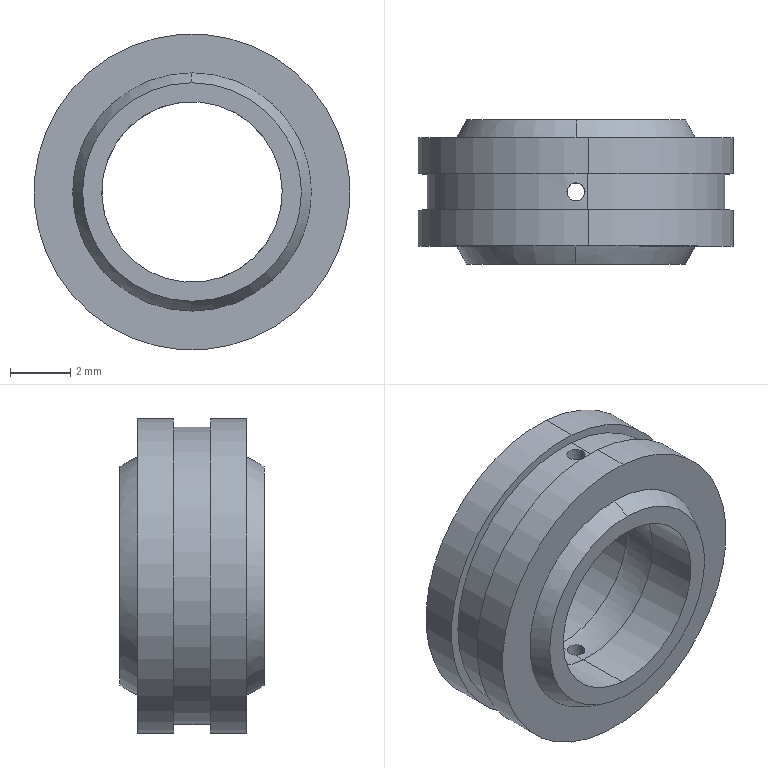Part | STEP file | 2026.6.15-Main Assembly图.sldasm-Part-227 | 1 solid | 29 faces | box 10.5 x 4.8 x 10.5 mm | volume 217.629 mm3 | cylinder 14 | plane 6 | torus 5 | sphere 4 | commonest cylinder face diameters 0.6 x4 6 x4 10.5 x4 9.9 x2
STEP:
#1=CARTESIAN_POINT('',(-1513.188,1424.864,3411.086));
#2=VERTEX_POINT('',#1);
#3=CARTESIAN_POINT('',(-1513.424,1424.864,3405.096));
#4=VERTEX_POINT('',#3);
#5=CARTESIAN_POINT('',(-1513.188,1424.864,3408.086));
#6=DIRECTION('',(0.,-1.,0.));
#7=DIRECTION('',(0.0785,0.,0.9969));
#8=AXIS2_PLACEMENT_3D('',#5,#6,#7);
#9=CIRCLE('',#8,3.);
#10=EDGE_CURVE('',#2,#4,#9,.T.);
#11=ORIENTED_EDGE('',*,*,#10,.F.);
#12=CARTESIAN_POINT('',(-1513.188,1424.564,3411.104));
#13=VERTEX_POINT('',#12);
#14=CARTESIAN_POINT('',(-1513.188,1424.264,3403.323));
#15=DIRECTION('',(1.,0.,0.));
#16=DIRECTION('',(0.,1.,0.));
#17=AXIS2_PLACEMENT_3D('',#14,#15,#16);
#18=CIRCLE('',#17,7.786);
#19=EDGE_CURVE('',#2,#13,#18,.T.);
#20=ORIENTED_EDGE('',*,*,#19,.T.);
#21=CARTESIAN_POINT('',(-1513.488,1424.264,3411.095));
#22=VERTEX_POINT('',#21);
#23=CARTESIAN_POINT('',(-1513.188,1424.564,3411.104));
#24=CARTESIAN_POINT('',(-1513.267,1424.564,3411.104));
#25=CARTESIAN_POINT('',(-1513.344,1424.532,3411.102));
#26=CARTESIAN_POINT('',(-1513.456,1424.421,3411.097));
#27=CARTESIAN_POINT('',(-1513.488,1424.344,3411.095));
#28=CARTESIAN_POINT('',(-1513.488,1424.264,3411.095));
#29=B_SPLINE_CURVE_WITH_KNOTS('',3,(#23,#24,#25,#26,#27,#28),.UNSPECIFIED.,.F.,.F.,(4,2,4),(0.0002723,0.0005067,0.0007411),.UNSPECIFIED.);
#30=EDGE_CURVE('',#13,#22,#29,.T.);
#31=ORIENTED_EDGE('',*,*,#30,.T.);
#32=CARTESIAN_POINT('',(-1513.188,1423.964,3411.104));
#33=VERTEX_POINT('',#32);
#34=CARTESIAN_POINT('',(-1513.488,1424.264,3411.095));
#35=CARTESIAN_POINT('',(-1513.488,1424.185,3411.095));
#36=CARTESIAN_POINT('',(-1513.456,1424.107,3411.097));
#37=CARTESIAN_POINT('',(-1513.345,1423.997,3411.102));
#38=CARTESIAN_POINT('',(-1513.267,1423.964,3411.104));
#39=CARTESIAN_POINT('',(-1513.188,1423.964,3411.104));
#40=B_SPLINE_CURVE_WITH_KNOTS('',3,(#34,#35,#36,#37,#38,#39),.UNSPECIFIED.,.F.,.F.,(4,2,4),(0.,0.0002346,0.0004692),.UNSPECIFIED.);
#41=EDGE_CURVE('',#22,#33,#40,.T.);
#42=ORIENTED_EDGE('',*,*,#41,.T.);
#43=CARTESIAN_POINT('',(-1513.188,1423.664,3411.086));
#44=VERTEX_POINT('',#43);
#45=CARTESIAN_POINT('',(-1513.188,1424.264,3403.323));
#46=DIRECTION('',(1.,0.,0.));
#47=DIRECTION('',(0.,1.,0.));
#48=AXIS2_PLACEMENT_3D('',#45,#46,#47);
#49=CIRCLE('',#48,7.786);
#50=EDGE_CURVE('',#33,#44,#49,.T.);
#51=ORIENTED_EDGE('',*,*,#50,.T.);
#52=CARTESIAN_POINT('',(-1513.424,1423.664,3405.096));
#53=VERTEX_POINT('',#52);
#54=CARTESIAN_POINT('',(-1513.188,1423.664,3408.086));
#55=DIRECTION('',(0.,-1.,0.));
#56=DIRECTION('',(-0.0785,0.,-0.9969));
#57=AXIS2_PLACEMENT_3D('',#54,#55,#56);
#58=CIRCLE('',#57,3.);
#59=EDGE_CURVE('',#44,#53,#58,.T.);
#60=ORIENTED_EDGE('',*,*,#59,.T.);
#61=CARTESIAN_POINT('',(-1513.425,1424.081,3405.075));
#62=VERTEX_POINT('',#61);
#63=CARTESIAN_POINT('',(-1512.814,1424.264,3412.835));
#64=DIRECTION('',(-0.9969,0.,0.0785));
#65=DIRECTION('',(-0.0785,0.,-0.9969));
#66=AXIS2_PLACEMENT_3D('',#63,#64,#65);
#67=CIRCLE('',#66,7.786);
#68=EDGE_CURVE('',#62,#53,#67,.T.);
#69=ORIENTED_EDGE('',*,*,#68,.F.);
#70=CARTESIAN_POINT('',(-1513.488,1424.264,3405.078));
#71=VERTEX_POINT('',#70);
#72=CARTESIAN_POINT('',(-1513.425,1424.081,3405.075));
#73=CARTESIAN_POINT('',(-1513.466,1424.133,3405.077));
#74=CARTESIAN_POINT('',(-1513.488,1424.198,3405.078));
#75=CARTESIAN_POINT('',(-1513.488,1424.264,3405.078));
#76=B_SPLINE_CURVE_WITH_KNOTS('',3,(#72,#73,#74,#75),.UNSPECIFIED.,.F.,.F.,(4,4),(0.,0.0001968),.UNSPECIFIED.);
#77=EDGE_CURVE('',#62,#71,#76,.T.);
#78=ORIENTED_EDGE('',*,*,#77,.T.);
#79=CARTESIAN_POINT('',(-1513.425,1424.448,3405.075));
#80=VERTEX_POINT('',#79);
#81=CARTESIAN_POINT('',(-1513.488,1424.264,3405.078));
#82=CARTESIAN_POINT('',(-1513.488,1424.331,3405.078));
#83=CARTESIAN_POINT('',(-1513.466,1424.395,3405.077));
#84=CARTESIAN_POINT('',(-1513.425,1424.448,3405.075));
#85=B_SPLINE_CURVE_WITH_KNOTS('',3,(#81,#82,#83,#84),.UNSPECIFIED.,.F.,.F.,(4,4),(0.,0.0001968),.UNSPECIFIED.);
#86=EDGE_CURVE('',#71,#80,#85,.T.);
#87=ORIENTED_EDGE('',*,*,#86,.T.);
#88=CARTESIAN_POINT('',(-1512.814,1424.264,3412.835));
#89=DIRECTION('',(-0.9969,0.,0.0785));
#90=DIRECTION('',(-0.0785,0.,-0.9969));
#91=AXIS2_PLACEMENT_3D('',#88,#89,#90);
#92=CIRCLE('',#91,7.786);
#93=EDGE_CURVE('',#4,#80,#92,.T.);
#94=ORIENTED_EDGE('',*,*,#93,.F.);
#95=EDGE_LOOP('',(#11,#20,#31,#42,#51,#60,#69,#78,#87,#94));
#96=FACE_OUTER_BOUND('',#95,.T.);
#97=CARTESIAN_POINT('',(-1513.188,1424.264,3408.086));
#98=DIRECTION('',(0.,-1.,0.));
#99=DIRECTION('',(0.,0.,1.));
#100=AXIS2_PLACEMENT_3D('',#97,#98,#99);
#101=TOROIDAL_SURFACE('',#100,-4.763,7.786);
#102=ADVANCED_FACE('',(#96),#101,.F.);
#103=ORIENTED_EDGE('',*,*,#19,.F.);
#104=CARTESIAN_POINT('',(-1512.953,1424.864,3411.077));
#105=VERTEX_POINT('',#104);
#106=CARTESIAN_POINT('',(-1513.188,1424.864,3408.086));
#107=DIRECTION('',(0.,-1.,0.));
#108=DIRECTION('',(0.0785,0.,0.9969));
#109=AXIS2_PLACEMENT_3D('',#106,#107,#108);
#110=CIRCLE('',#109,3.);
#111=EDGE_CURVE('',#105,#2,#110,.T.);
#112=ORIENTED_EDGE('',*,*,#111,.F.);
#113=CARTESIAN_POINT('',(-1512.951,1424.448,3411.098));
#114=VERTEX_POINT('',#113);
#115=CARTESIAN_POINT('',(-1513.562,1424.264,3403.338));
#116=DIRECTION('',(0.9969,0.,-0.0785));
#117=DIRECTION('',(0.0785,0.,0.9969));
#118=AXIS2_PLACEMENT_3D('',#115,#116,#117);
#119=CIRCLE('',#118,7.786);
#120=EDGE_CURVE('',#105,#114,#119,.T.);
#121=ORIENTED_EDGE('',*,*,#120,.T.);
#122=CARTESIAN_POINT('',(-1512.951,1424.448,3411.098));
#123=CARTESIAN_POINT('',(-1513.008,1424.521,3411.101));
#124=CARTESIAN_POINT('',(-1513.097,1424.564,3411.104));
#125=CARTESIAN_POINT('',(-1513.188,1424.564,3411.104));
#126=B_SPLINE_CURVE_WITH_KNOTS('',3,(#122,#123,#124,#125),.UNSPECIFIED.,.F.,.F.,(4,4),(0.,0.0002723),.UNSPECIFIED.);
#127=EDGE_CURVE('',#114,#13,#126,.T.);
#128=ORIENTED_EDGE('',*,*,#127,.T.);
#129=EDGE_LOOP('',(#103,#112,#121,#128));
#130=FACE_OUTER_BOUND('',#129,.T.);
#131=CARTESIAN_POINT('',(-1513.188,1424.264,3408.086));
#132=DIRECTION('',(0.,-1.,0.));
#133=DIRECTION('',(0.,0.,1.));
#134=AXIS2_PLACEMENT_3D('',#131,#132,#133);
#135=TOROIDAL_SURFACE('',#134,-4.763,7.786);
#136=ADVANCED_FACE('',(#130),#135,.F.);
#137=CARTESIAN_POINT('',(-1510.188,1424.864,3408.086));
#138=VERTEX_POINT('',#137);
#139=CARTESIAN_POINT('',(-1513.188,1424.864,3408.086));
#140=DIRECTION('',(0.,-1.,0.));
#141=DIRECTION('',(0.0785,0.,0.9969));
#142=AXIS2_PLACEMENT_3D('',#139,#140,#141);
#143=CIRCLE('',#142,3.);
#144=EDGE_CURVE('',#138,#105,#143,.T.);
#145=ORIENTED_EDGE('',*,*,#144,.F.);
#146=CARTESIAN_POINT('',(-1510.188,1423.664,3408.086));
#147=VERTEX_POINT('',#146);
#148=CARTESIAN_POINT('',(-1517.951,1424.264,3408.086));
#149=DIRECTION('',(0.,0.,-1.));
#150=DIRECTION('',(0.,1.,0.));
#151=AXIS2_PLACEMENT_3D('',#148,#149,#150);
#152=CIRCLE('',#151,7.786);
#153=EDGE_CURVE('',#138,#147,#152,.T.);
#154=ORIENTED_EDGE('',*,*,#153,.T.);
#155=CARTESIAN_POINT('',(-1512.953,1423.664,3411.077));
#156=VERTEX_POINT('',#155);
#157=CARTESIAN_POINT('',(-1513.188,1423.664,3408.086));
#158=DIRECTION('',(0.,-1.,0.));
#159=DIRECTION('',(-0.0785,0.,-0.9969));
#160=AXIS2_PLACEMENT_3D('',#157,#158,#159);
#161=CIRCLE('',#160,3.);
#162=EDGE_CURVE('',#147,#156,#161,.T.);
#163=ORIENTED_EDGE('',*,*,#162,.T.);
#164=CARTESIAN_POINT('',(-1512.951,1424.081,3411.098));
#165=VERTEX_POINT('',#164);
#166=CARTESIAN_POINT('',(-1513.562,1424.264,3403.338));
#167=DIRECTION('',(0.9969,0.,-0.0785));
#168=DIRECTION('',(0.0785,0.,0.9969));
#169=AXIS2_PLACEMENT_3D('',#166,#167,#168);
#170=CIRCLE('',#169,7.786);
#171=EDGE_CURVE('',#165,#156,#170,.T.);
#172=ORIENTED_EDGE('',*,*,#171,.F.);
#173=CARTESIAN_POINT('',(-1512.888,1424.264,3411.095));
#174=VERTEX_POINT('',#173);
#175=CARTESIAN_POINT('',(-1512.951,1424.081,3411.098));
#176=CARTESIAN_POINT('',(-1512.91,1424.133,3411.096));
#177=CARTESIAN_POINT('',(-1512.888,1424.198,3411.095));
#178=CARTESIAN_POINT('',(-1512.888,1424.264,3411.095));
#179=B_SPLINE_CURVE_WITH_KNOTS('',3,(#175,#176,#177,#178),.UNSPECIFIED.,.F.,.F.,(4,4),(0.,0.0001968),.UNSPECIFIED.);
#180=EDGE_CURVE('',#165,#174,#179,.T.);
#181=ORIENTED_EDGE('',*,*,#180,.T.);
#182=CARTESIAN_POINT('',(-1512.888,1424.264,3411.095));
#183=CARTESIAN_POINT('',(-1512.888,1424.331,3411.095));
#184=CARTESIAN_POINT('',(-1512.91,1424.395,3411.096));
#185=CARTESIAN_POINT('',(-1512.951,1424.448,3411.098));
#186=B_SPLINE_CURVE_WITH_KNOTS('',3,(#182,#183,#184,#185),.UNSPECIFIED.,.F.,.F.,(4,4),(0.,0.0001968),.UNSPECIFIED.);
#187=EDGE_CURVE('',#174,#114,#186,.T.);
#188=ORIENTED_EDGE('',*,*,#187,.T.);
#189=ORIENTED_EDGE('',*,*,#120,.F.);
#190=EDGE_LOOP('',(#145,#154,#163,#172,#181,#188,#189));
#191=FACE_OUTER_BOUND('',#190,.T.);
#192=CARTESIAN_POINT('',(-1513.188,1424.264,3408.086));
#193=DIRECTION('',(0.,-1.,0.));
#194=DIRECTION('',(1.,0.,0.));
#195=AXIS2_PLACEMENT_3D('',#192,#193,#194);
#196=TOROIDAL_SURFACE('',#195,-4.763,7.786);
#197=ADVANCED_FACE('',(#191),#196,.F.);
#198=CARTESIAN_POINT('',(-1513.188,1422.464,3412.046));
#199=VERTEX_POINT('',#198);
#200=CARTESIAN_POINT('',(-1513.188,1422.464,3404.126));
#201=VERTEX_POINT('',#200);
#202=CARTESIAN_POINT('',(-1513.188,1422.464,3408.086));
#203=DIRECTION('',(0.,1.,0.));
#204=DIRECTION('',(0.0785,0.,0.9969));
#205=AXIS2_PLACEMENT_3D('',#202,#203,#204);
#206=CIRCLE('',#205,3.96);
#207=EDGE_CURVE('',#199,#201,#206,.T.);
#208=ORIENTED_EDGE('',*,*,#207,.F.);
#209=CARTESIAN_POINT('',(-1513.188,1421.864,3411.714));
#210=VERTEX_POINT('',#209);
#211=CARTESIAN_POINT('',(-1513.188,1424.264,3408.086));
#212=DIRECTION('',(-1.,0.,0.));
#213=DIRECTION('',(0.,-1.,0.));
#214=AXIS2_PLACEMENT_3D('',#211,#212,#213);
#215=CIRCLE('',#214,4.35);
#216=EDGE_CURVE('',#210,#199,#215,.T.);
#217=ORIENTED_EDGE('',*,*,#216,.F.);
#218=CARTESIAN_POINT('',(-1513.188,1421.864,3404.458));
#219=VERTEX_POINT('',#218);
#220=CARTESIAN_POINT('',(-1513.188,1421.864,3408.086));
#221=DIRECTION('',(0.,1.,0.));
#222=DIRECTION('',(0.0785,0.,0.9969));
#223=AXIS2_PLACEMENT_3D('',#220,#221,#222);
#224=CIRCLE('',#223,3.628);
#225=EDGE_CURVE('',#210,#219,#224,.T.);
#226=ORIENTED_EDGE('',*,*,#225,.T.);
#227=CARTESIAN_POINT('',(-1513.188,1424.264,3408.086));
#228=DIRECTION('',(1.,0.,0.));
#229=DIRECTION('',(0.,1.,0.));
#230=AXIS2_PLACEMENT_3D('',#227,#228,#229);
#231=CIRCLE('',#230,4.35);
#232=EDGE_CURVE('',#219,#201,#231,.T.);
#233=ORIENTED_EDGE('',*,*,#232,.T.);
#234=EDGE_LOOP('',(#208,#217,#226,#233));
#235=FACE_OUTER_BOUND('',#234,.T.);
#236=CARTESIAN_POINT('',(-1513.188,1424.264,3408.086));
#237=DIRECTION('',(1.,0.,0.));
#238=DIRECTION('',(0.,0.4075,0.9132));
#239=AXIS2_PLACEMENT_3D('',#236,#237,#238);
#240=SPHERICAL_SURFACE('',#239,4.35);
#241=ADVANCED_FACE('',(#235),#240,.T.);
#242=CARTESIAN_POINT('',(-1513.188,1426.064,3404.126));
#243=VERTEX_POINT('',#242);
#244=CARTESIAN_POINT('',(-1513.188,1426.064,3412.046));
#245=VERTEX_POINT('',#244);
#246=CARTESIAN_POINT('',(-1513.188,1426.064,3408.086));
#247=DIRECTION('',(0.,-1.,0.));
#248=DIRECTION('',(-0.0785,0.,-0.9969));
#249=AXIS2_PLACEMENT_3D('',#246,#247,#248);
#250=CIRCLE('',#249,3.96);
#251=EDGE_CURVE('',#243,#245,#250,.T.);
#252=ORIENTED_EDGE('',*,*,#251,.F.);
#253=CARTESIAN_POINT('',(-1513.188,1426.664,3404.458));
#254=VERTEX_POINT('',#253);
#255=CARTESIAN_POINT('',(-1513.188,1424.264,3408.086));
#256=DIRECTION('',(1.,0.,0.));
#257=DIRECTION('',(0.,0.,-1.));
#258=AXIS2_PLACEMENT_3D('',#255,#256,#257);
#259=CIRCLE('',#258,4.35);
#260=EDGE_CURVE('',#243,#254,#259,.T.);
#261=ORIENTED_EDGE('',*,*,#260,.T.);
#262=CARTESIAN_POINT('',(-1513.188,1426.664,3411.714));
#263=VERTEX_POINT('',#262);
#264=CARTESIAN_POINT('',(-1513.188,1426.664,3408.086));
#265=DIRECTION('',(0.,1.,0.));
#266=DIRECTION('',(-0.0785,0.,-0.9969));
#267=AXIS2_PLACEMENT_3D('',#264,#265,#266);
#268=CIRCLE('',#267,3.628);
#269=EDGE_CURVE('',#263,#254,#268,.T.);
#270=ORIENTED_EDGE('',*,*,#269,.F.);
#271=CARTESIAN_POINT('',(-1513.188,1424.264,3408.086));
#272=DIRECTION('',(-1.,0.,0.));
#273=DIRECTION('',(0.,0.,1.));
#274=AXIS2_PLACEMENT_3D('',#271,#272,#273);
#275=CIRCLE('',#274,4.35);
#276=EDGE_CURVE('',#245,#263,#275,.T.);
#277=ORIENTED_EDGE('',*,*,#276,.F.);
#278=EDGE_LOOP('',(#252,#261,#270,#277));
#279=FACE_OUTER_BOUND('',#278,.T.);
#280=CARTESIAN_POINT('',(-1513.188,1424.264,3408.086));
#281=DIRECTION('',(1.,0.,0.));
#282=DIRECTION('',(0.,-0.4012,-0.916));
#283=AXIS2_PLACEMENT_3D('',#280,#281,#282);
#284=SPHERICAL_SURFACE('',#283,4.35);
#285=ADVANCED_FACE('',(#279),#284,.T.);
#286=ORIENTED_EDGE('',*,*,#260,.F.);
#287=CARTESIAN_POINT('',(-1513.188,1426.064,3408.086));
#288=DIRECTION('',(0.,-1.,0.));
#289=DIRECTION('',(-0.0785,0.,-0.9969));
#290=AXIS2_PLACEMENT_3D('',#287,#288,#289);
#291=CIRCLE('',#290,3.96);
#292=EDGE_CURVE('',#245,#243,#291,.T.);
#293=ORIENTED_EDGE('',*,*,#292,.F.);
#294=ORIENTED_EDGE('',*,*,#276,.T.);
#295=CARTESIAN_POINT('',(-1513.188,1426.664,3408.086));
#296=DIRECTION('',(0.,1.,0.));
#297=DIRECTION('',(-0.0785,0.,-0.9969));
#298=AXIS2_PLACEMENT_3D('',#295,#296,#297);
#299=CIRCLE('',#298,3.628);
#300=EDGE_CURVE('',#254,#263,#299,.T.);
#301=ORIENTED_EDGE('',*,*,#300,.F.);
#302=EDGE_LOOP('',(#286,#293,#294,#301));
#303=FACE_OUTER_BOUND('',#302,.T.);
#304=CARTESIAN_POINT('',(-1513.188,1424.264,3408.086));
#305=DIRECTION('',(1.,0.,0.));
#306=DIRECTION('',(0.,-0.4012,-0.916));
#307=AXIS2_PLACEMENT_3D('',#304,#305,#306);
#308=SPHERICAL_SURFACE('',#307,4.35);
#309=ADVANCED_FACE('',(#303),#308,.T.);
#310=ORIENTED_EDGE('',*,*,#269,.T.);
#311=ORIENTED_EDGE('',*,*,#300,.T.);
#312=EDGE_LOOP('',(#310,#311));
#313=FACE_OUTER_BOUND('',#312,.T.);
#314=CARTESIAN_POINT('',(-1513.424,1426.664,3405.096));
#315=VERTEX_POINT('',#314);
#316=CARTESIAN_POINT('',(-1512.953,1426.664,3411.077));
#317=VERTEX_POINT('',#316);
#318=CARTESIAN_POINT('',(-1513.188,1426.664,3408.086));
#319=DIRECTION('',(0.,-1.,0.));
#320=DIRECTION('',(-0.0785,0.,-0.9969));
#321=AXIS2_PLACEMENT_3D('',#318,#319,#320);
#322=CIRCLE('',#321,3.);
#323=EDGE_CURVE('',#315,#317,#322,.T.);
#324=ORIENTED_EDGE('',*,*,#323,.T.);
#325=CARTESIAN_POINT('',(-1513.188,1426.664,3408.086));
#326=DIRECTION('',(0.,-1.,0.));
#327=DIRECTION('',(-0.0785,0.,-0.9969));
#328=AXIS2_PLACEMENT_3D('',#325,#326,#327);
#329=CIRCLE('',#328,3.);
#330=EDGE_CURVE('',#317,#315,#329,.T.);
#331=ORIENTED_EDGE('',*,*,#330,.T.);
#332=EDGE_LOOP('',(#324,#331));
#333=FACE_BOUND('',#332,.T.);
#334=CARTESIAN_POINT('',(-1513.188,1426.664,3408.086));
#335=DIRECTION('',(0.,1.,0.));
#336=DIRECTION('',(0.,0.,-1.));
#337=AXIS2_PLACEMENT_3D('',#334,#335,#336);
#338=PLANE('',#337);
#339=ADVANCED_FACE('',(#313,#333),#338,.T.);
#340=CARTESIAN_POINT('',(-1513.6,1426.064,3402.853));
#341=VERTEX_POINT('',#340);
#342=CARTESIAN_POINT('',(-1512.776,1426.064,3413.32));
#343=VERTEX_POINT('',#342);
#344=CARTESIAN_POINT('',(-1513.188,1426.064,3408.086));
#345=DIRECTION('',(0.,-1.,0.));
#346=DIRECTION('',(-0.0785,0.,-0.9969));
#347=AXIS2_PLACEMENT_3D('',#344,#345,#346);
#348=CIRCLE('',#347,5.25);
#349=EDGE_CURVE('',#341,#343,#348,.T.);
#350=ORIENTED_EDGE('',*,*,#349,.F.);
#351=CARTESIAN_POINT('',(-1513.188,1426.064,3408.086));
#352=DIRECTION('',(0.,-1.,0.));
#353=DIRECTION('',(-0.0785,0.,-0.9969));
#354=AXIS2_PLACEMENT_3D('',#351,#352,#353);
#355=CIRCLE('',#354,5.25);
#356=EDGE_CURVE('',#343,#341,#355,.T.);
#357=ORIENTED_EDGE('',*,*,#356,.F.);
#358=EDGE_LOOP('',(#350,#357));
#359=FACE_OUTER_BOUND('',#358,.T.);
#360=ORIENTED_EDGE('',*,*,#292,.T.);
#361=ORIENTED_EDGE('',*,*,#251,.T.);
#362=EDGE_LOOP('',(#360,#361));
#363=FACE_BOUND('',#362,.T.);
#364=CARTESIAN_POINT('',(-1513.188,1426.064,3413.336));
#365=DIRECTION('',(0.,1.,0.));
#366=DIRECTION('',(0.,0.,-1.));
#367=AXIS2_PLACEMENT_3D('',#364,#365,#366);
#368=PLANE('',#367);
#369=ADVANCED_FACE('',(#359,#363),#368,.T.);
#370=CARTESIAN_POINT('',(-1512.953,1406.264,3411.077));
#371=DIRECTION('',(0.,1.,0.));
#372=VECTOR('',#371,1000.);
#373=LINE('',#370,#372);
#374=EDGE_CURVE('',#105,#317,#373,.T.);
#375=ORIENTED_EDGE('',*,*,#374,.F.);
#376=ORIENTED_EDGE('',*,*,#111,.T.);
#377=ORIENTED_EDGE('',*,*,#10,.T.);
#378=CARTESIAN_POINT('',(-1513.424,1406.264,3405.096));
#379=DIRECTION('',(0.,1.,0.));
#380=VECTOR('',#379,1000.);
#381=LINE('',#378,#380);
#382=EDGE_CURVE('',#4,#315,#381,.T.);
#383=ORIENTED_EDGE('',*,*,#382,.T.);
#384=ORIENTED_EDGE('',*,*,#330,.F.);
#385=EDGE_LOOP('',(#375,#376,#377,#383,#384));
#386=FACE_OUTER_BOUND('',#385,.T.);
#387=CARTESIAN_POINT('',(-1513.188,1406.264,3408.086));
#388=DIRECTION('',(0.,1.,0.));
#389=DIRECTION('',(0.0785,0.,0.9969));
#390=AXIS2_PLACEMENT_3D('',#387,#388,#389);
#391=CYLINDRICAL_SURFACE('',#390,3.);
#392=ADVANCED_FACE('',(#386),#391,.F.);
#393=CARTESIAN_POINT('',(-1512.776,1424.864,3413.32));
#394=VERTEX_POINT('',#393);
#395=CARTESIAN_POINT('',(-1512.776,1406.264,3413.32));
#396=DIRECTION('',(0.,1.,0.));
#397=VECTOR('',#396,1000.);
#398=LINE('',#395,#397);
#399=EDGE_CURVE('',#394,#343,#398,.T.);
#400=ORIENTED_EDGE('',*,*,#399,.F.);
#401=CARTESIAN_POINT('',(-1513.6,1424.864,3402.853));
#402=VERTEX_POINT('',#401);
#403=CARTESIAN_POINT('',(-1513.188,1424.864,3408.086));
#404=DIRECTION('',(0.,-1.,0.));
#405=DIRECTION('',(-0.0785,0.,-0.9969));
#406=AXIS2_PLACEMENT_3D('',#403,#404,#405);
#407=CIRCLE('',#406,5.25);
#408=EDGE_CURVE('',#402,#394,#407,.T.);
#409=ORIENTED_EDGE('',*,*,#408,.F.);
#410=CARTESIAN_POINT('',(-1513.6,1406.264,3402.853));
#411=DIRECTION('',(0.,1.,0.));
#412=VECTOR('',#411,1000.);
#413=LINE('',#410,#412);
#414=EDGE_CURVE('',#402,#341,#413,.T.);
#415=ORIENTED_EDGE('',*,*,#414,.T.);
#416=ORIENTED_EDGE('',*,*,#349,.T.);
#417=EDGE_LOOP('',(#400,#409,#415,#416));
#418=FACE_OUTER_BOUND('',#417,.T.);
#419=CARTESIAN_POINT('',(-1513.188,1406.264,3408.086));
#420=DIRECTION('',(0.,1.,0.));
#421=DIRECTION('',(0.0785,0.,0.9969));
#422=AXIS2_PLACEMENT_3D('',#419,#420,#421);
#423=CYLINDRICAL_SURFACE('',#422,5.25);
#424=ADVANCED_FACE('',(#418),#423,.T.);
#425=ORIENTED_EDGE('',*,*,#153,.F.);
#426=CARTESIAN_POINT('',(-1513.188,1424.864,3408.086));
#427=DIRECTION('',(0.,-1.,0.));
#428=DIRECTION('',(0.0785,0.,0.9969));
#429=AXIS2_PLACEMENT_3D('',#426,#427,#428);
#430=CIRCLE('',#429,3.);
#431=EDGE_CURVE('',#4,#138,#430,.T.);
#432=ORIENTED_EDGE('',*,*,#431,.F.);
#433=ORIENTED_EDGE('',*,*,#93,.T.);
#434=CARTESIAN_POINT('',(-1512.888,1424.264,3405.078));
#435=VERTEX_POINT('',#434);
#436=CARTESIAN_POINT('',(-1513.425,1424.448,3405.075));
#437=CARTESIAN_POINT('',(-1513.387,1424.498,3405.073));
#438=CARTESIAN_POINT('',(-1513.334,1424.534,3405.071));
#439=CARTESIAN_POINT('',(-1513.215,1424.57,3405.069));
#440=CARTESIAN_POINT('',(-1513.15,1424.568,3405.069));
#441=CARTESIAN_POINT('',(-1513.033,1424.528,3405.071));
#442=CARTESIAN_POINT('',(-1512.98,1424.489,3405.073));
#443=CARTESIAN_POINT('',(-1512.908,1424.389,3405.077));
#444=CARTESIAN_POINT('',(-1512.888,1424.327,3405.078));
#445=CARTESIAN_POINT('',(-1512.888,1424.264,3405.078));
#446=B_SPLINE_CURVE_WITH_KNOTS('',3,(#436,#437,#438,#439,#440,#441,#442,#443,#444,#445),.UNSPECIFIED.,.F.,.F.,(4,2,2,2,4),(0.,0.0001853,0.0003705,0.0005558,0.0007411),.UNSPECIFIED.);
#447=EDGE_CURVE('',#80,#435,#446,.T.);
#448=ORIENTED_EDGE('',*,*,#447,.T.);
#449=CARTESIAN_POINT('',(-1512.888,1424.264,3405.078));
#450=CARTESIAN_POINT('',(-1512.888,1424.202,3405.078));
#451=CARTESIAN_POINT('',(-1512.908,1424.141,3405.077));
#452=CARTESIAN_POINT('',(-1512.98,1424.039,3405.073));
#453=CARTESIAN_POINT('',(-1513.032,1424.001,3405.071));
#454=CARTESIAN_POINT('',(-1513.149,1423.96,3405.069));
#455=CARTESIAN_POINT('',(-1513.215,1423.959,3405.069));
#456=CARTESIAN_POINT('',(-1513.333,1423.995,3405.071));
#457=CARTESIAN_POINT('',(-1513.387,1424.031,3405.073));
#458=CARTESIAN_POINT('',(-1513.425,1424.081,3405.075));
#459=B_SPLINE_CURVE_WITH_KNOTS('',3,(#449,#450,#451,#452,#453,#454,#455,#456,#457,#458),.UNSPECIFIED.,.F.,.F.,(4,2,2,2,4),(0.,0.0001853,0.0003705,0.0005558,0.000741),.UNSPECIFIED.);
#460=EDGE_CURVE('',#435,#62,#459,.T.);
#461=ORIENTED_EDGE('',*,*,#460,.T.);
#462=ORIENTED_EDGE('',*,*,#68,.T.);
#463=CARTESIAN_POINT('',(-1513.188,1423.664,3408.086));
#464=DIRECTION('',(0.,-1.,0.));
#465=DIRECTION('',(-0.0785,0.,-0.9969));
#466=AXIS2_PLACEMENT_3D('',#463,#464,#465);
#467=CIRCLE('',#466,3.);
#468=EDGE_CURVE('',#53,#147,#467,.T.);
#469=ORIENTED_EDGE('',*,*,#468,.T.);
#470=EDGE_LOOP('',(#425,#432,#433,#448,#461,#462,#469));
#471=FACE_OUTER_BOUND('',#470,.T.);
#472=CARTESIAN_POINT('',(-1513.188,1424.264,3408.086));
#473=DIRECTION('',(0.,-1.,0.));
#474=DIRECTION('',(1.,0.,0.));
#475=AXIS2_PLACEMENT_3D('',#472,#473,#474);
#476=TOROIDAL_SURFACE('',#475,-4.763,7.786);
#477=ADVANCED_FACE('',(#471),#476,.F.);
#478=CARTESIAN_POINT('',(-1512.888,1424.264,3413.027));
#479=VERTEX_POINT('',#478);
#480=CARTESIAN_POINT('',(-1512.888,1424.264,3397.731));
#481=DIRECTION('',(0.,0.,1.));
#482=VECTOR('',#481,1000.);
#483=LINE('',#480,#482);
#484=EDGE_CURVE('',#174,#479,#483,.T.);
#485=ORIENTED_EDGE('',*,*,#484,.T.);
#486=CARTESIAN_POINT('',(-1513.488,1424.264,3413.027));
#487=VERTEX_POINT('',#486);
#488=CARTESIAN_POINT('',(-1513.488,1424.264,3413.027));
#489=CARTESIAN_POINT('',(-1513.488,1424.344,3413.027));
#490=CARTESIAN_POINT('',(-1513.456,1424.421,3413.029));
#491=CARTESIAN_POINT('',(-1513.345,1424.532,3413.034));
#492=CARTESIAN_POINT('',(-1513.267,1424.564,3413.036));
#493=CARTESIAN_POINT('',(-1513.11,1424.564,3413.036));
#494=CARTESIAN_POINT('',(-1513.032,1424.533,3413.034));
#495=CARTESIAN_POINT('',(-1512.92,1424.421,3413.029));
#496=CARTESIAN_POINT('',(-1512.888,1424.344,3413.027));
#497=CARTESIAN_POINT('',(-1512.888,1424.264,3413.027));
#498=B_SPLINE_CURVE_WITH_KNOTS('',3,(#488,#489,#490,#491,#492,#493,#494,#495,#496,#497),.UNSPECIFIED.,.F.,.F.,(4,2,2,2,4),(0.,0.0002345,0.000469,0.0007035,0.000938),.UNSPECIFIED.);
#499=EDGE_CURVE('',#487,#479,#498,.T.);
#500=ORIENTED_EDGE('',*,*,#499,.F.);
#501=CARTESIAN_POINT('',(-1513.488,1424.264,3397.731));
#502=DIRECTION('',(0.,0.,1.));
#503=VECTOR('',#502,1000.);
#504=LINE('',#501,#503);
#505=EDGE_CURVE('',#22,#487,#504,.T.);
#506=ORIENTED_EDGE('',*,*,#505,.F.);
#507=ORIENTED_EDGE('',*,*,#30,.F.);
#508=ORIENTED_EDGE('',*,*,#127,.F.);
#509=ORIENTED_EDGE('',*,*,#187,.F.);
#510=EDGE_LOOP('',(#485,#500,#506,#507,#508,#509));
#511=FACE_OUTER_BOUND('',#510,.T.);
#512=CARTESIAN_POINT('',(-1513.188,1424.264,3397.731));
#513=DIRECTION('',(0.,0.,-1.));
#514=DIRECTION('',(1.,0.,0.));
#515=AXIS2_PLACEMENT_3D('',#512,#513,#514);
#516=CYLINDRICAL_SURFACE('',#515,0.3);
#517=ADVANCED_FACE('',(#511),#516,.F.);
#518=ORIENTED_EDGE('',*,*,#408,.T.);
#519=CARTESIAN_POINT('',(-1513.188,1424.864,3408.086));
#520=DIRECTION('',(0.,-1.,0.));
#521=DIRECTION('',(-0.0785,0.,-0.9969));
#522=AXIS2_PLACEMENT_3D('',#519,#520,#521);
#523=CIRCLE('',#522,5.25);
#524=EDGE_CURVE('',#394,#402,#523,.T.);
#525=ORIENTED_EDGE('',*,*,#524,.T.);
#526=EDGE_LOOP('',(#518,#525));
#527=FACE_OUTER_BOUND('',#526,.T.);
#528=CARTESIAN_POINT('',(-1513.577,1424.864,3403.152));
#529=VERTEX_POINT('',#528);
#530=CARTESIAN_POINT('',(-1512.8,1424.864,3413.021));
#531=VERTEX_POINT('',#530);
#532=CARTESIAN_POINT('',(-1513.188,1424.864,3408.086));
#533=DIRECTION('',(0.,-1.,0.));
#534=DIRECTION('',(-0.0785,0.,-0.9969));
#535=AXIS2_PLACEMENT_3D('',#532,#533,#534);
#536=CIRCLE('',#535,4.95);
#537=EDGE_CURVE('',#529,#531,#536,.T.);
#538=ORIENTED_EDGE('',*,*,#537,.F.);
#539=CARTESIAN_POINT('',(-1513.188,1424.864,3408.086));
#540=DIRECTION('',(0.,-1.,0.));
#541=DIRECTION('',(-0.0785,0.,-0.9969));
#542=AXIS2_PLACEMENT_3D('',#539,#540,#541);
#543=CIRCLE('',#542,4.95);
#544=EDGE_CURVE('',#531,#529,#543,.T.);
#545=ORIENTED_EDGE('',*,*,#544,.F.);
#546=EDGE_LOOP('',(#538,#545));
#547=FACE_BOUND('',#546,.T.);
#548=CARTESIAN_POINT('',(-1513.188,1424.864,3413.036));
#549=DIRECTION('',(0.,-1.,0.));
#550=DIRECTION('',(-1.,0.,0.));
#551=AXIS2_PLACEMENT_3D('',#548,#549,#550);
#552=PLANE('',#551);
#553=ADVANCED_FACE('',(#527,#547),#552,.T.);
#554=CARTESIAN_POINT('',(-1512.888,1424.264,3403.145));
#555=VERTEX_POINT('',#554);
#556=CARTESIAN_POINT('',(-1512.888,1424.264,3397.731));
#557=DIRECTION('',(0.,0.,1.));
#558=VECTOR('',#557,1000.);
#559=LINE('',#556,#558);
#560=EDGE_CURVE('',#555,#435,#559,.T.);
#561=ORIENTED_EDGE('',*,*,#560,.T.);
#562=ORIENTED_EDGE('',*,*,#447,.F.);
#563=ORIENTED_EDGE('',*,*,#86,.F.);
#564=CARTESIAN_POINT('',(-1513.488,1424.264,3403.145));
#565=VERTEX_POINT('',#564);
#566=CARTESIAN_POINT('',(-1513.488,1424.264,3397.731));
#567=DIRECTION('',(0.,0.,1.));
#568=VECTOR('',#567,1000.);
#569=LINE('',#566,#568);
#570=EDGE_CURVE('',#565,#71,#569,.T.);
#571=ORIENTED_EDGE('',*,*,#570,.F.);
#572=CARTESIAN_POINT('',(-1512.888,1424.264,3403.145));
#573=CARTESIAN_POINT('',(-1512.888,1424.344,3403.145));
#574=CARTESIAN_POINT('',(-1512.921,1424.421,3403.143));
#575=CARTESIAN_POINT('',(-1513.031,1424.532,3403.139));
#576=CARTESIAN_POINT('',(-1513.11,1424.564,3403.136));
#577=CARTESIAN_POINT('',(-1513.266,1424.564,3403.136));
#578=CARTESIAN_POINT('',(-1513.344,1424.533,3403.138));
#579=CARTESIAN_POINT('',(-1513.456,1424.421,3403.143));
#580=CARTESIAN_POINT('',(-1513.488,1424.344,3403.145));
#581=CARTESIAN_POINT('',(-1513.488,1424.264,3403.145));
#582=B_SPLINE_CURVE_WITH_KNOTS('',3,(#572,#573,#574,#575,#576,#577,#578,#579,#580,#581),.UNSPECIFIED.,.F.,.F.,(4,2,2,2,4),(0.,0.0002345,0.000469,0.0007035,0.000938),.UNSPECIFIED.);
#583=EDGE_CURVE('',#555,#565,#582,.T.);
#584=ORIENTED_EDGE('',*,*,#583,.F.);
#585=EDGE_LOOP('',(#561,#562,#563,#571,#584));
#586=FACE_OUTER_BOUND('',#585,.T.);
#587=CARTESIAN_POINT('',(-1513.188,1424.264,3397.731));
#588=DIRECTION('',(0.,0.,-1.));
#589=DIRECTION('',(1.,0.,0.));
#590=AXIS2_PLACEMENT_3D('',#587,#588,#589);
#591=CYLINDRICAL_SURFACE('',#590,0.3);
#592=ADVANCED_FACE('',(#586),#591,.F.);
#593=CARTESIAN_POINT('',(-1512.953,1421.864,3411.077));
#594=VERTEX_POINT('',#593);
#595=CARTESIAN_POINT('',(-1512.953,1406.264,3411.077));
#596=DIRECTION('',(0.,1.,0.));
#597=VECTOR('',#596,1000.);
#598=LINE('',#595,#597);
#599=EDGE_CURVE('',#594,#156,#598,.T.);
#600=ORIENTED_EDGE('',*,*,#599,.F.);
#601=CARTESIAN_POINT('',(-1513.424,1421.864,3405.096));
#602=VERTEX_POINT('',#601);
#603=CARTESIAN_POINT('',(-1513.188,1421.864,3408.086));
#604=DIRECTION('',(0.,1.,0.));
#605=DIRECTION('',(-0.0785,0.,-0.9969));
#606=AXIS2_PLACEMENT_3D('',#603,#604,#605);
#607=CIRCLE('',#606,3.);
#608=EDGE_CURVE('',#602,#594,#607,.T.);
#609=ORIENTED_EDGE('',*,*,#608,.F.);
#610=CARTESIAN_POINT('',(-1513.424,1406.264,3405.096));
#611=DIRECTION('',(0.,1.,0.));
#612=VECTOR('',#611,1000.);
#613=LINE('',#610,#612);
#614=EDGE_CURVE('',#602,#53,#613,.T.);
#615=ORIENTED_EDGE('',*,*,#614,.T.);
#616=ORIENTED_EDGE('',*,*,#59,.F.);
#617=CARTESIAN_POINT('',(-1513.188,1423.664,3408.086));
#618=DIRECTION('',(0.,-1.,0.));
#619=DIRECTION('',(-0.0785,0.,-0.9969));
#620=AXIS2_PLACEMENT_3D('',#617,#618,#619);
#621=CIRCLE('',#620,3.);
#622=EDGE_CURVE('',#156,#44,#621,.T.);
#623=ORIENTED_EDGE('',*,*,#622,.F.);
#624=EDGE_LOOP('',(#600,#609,#615,#616,#623));
#625=FACE_OUTER_BOUND('',#624,.T.);
#626=CARTESIAN_POINT('',(-1513.188,1406.264,3408.086));
#627=DIRECTION('',(0.,1.,0.));
#628=DIRECTION('',(0.0785,0.,0.9969));
#629=AXIS2_PLACEMENT_3D('',#626,#627,#628);
#630=CYLINDRICAL_SURFACE('',#629,3.);
#631=ADVANCED_FACE('',(#625),#630,.F.);
#632=CARTESIAN_POINT('',(-1512.8,1423.664,3413.021));
#633=VERTEX_POINT('',#632);
#634=CARTESIAN_POINT('',(-1512.8,1406.264,3413.021));
#635=DIRECTION('',(0.,1.,0.));
#636=VECTOR('',#635,1000.);
#637=LINE('',#634,#636);
#638=EDGE_CURVE('',#633,#531,#637,.T.);
#639=ORIENTED_EDGE('',*,*,#638,.F.);
#640=CARTESIAN_POINT('',(-1513.577,1423.664,3403.152));
#641=VERTEX_POINT('',#640);
#642=CARTESIAN_POINT('',(-1513.188,1423.664,3408.086));
#643=DIRECTION('',(0.,-1.,0.));
#644=DIRECTION('',(-0.0785,0.,-0.9969));
#645=AXIS2_PLACEMENT_3D('',#642,#643,#644);
#646=CIRCLE('',#645,4.95);
#647=EDGE_CURVE('',#641,#633,#646,.T.);
#648=ORIENTED_EDGE('',*,*,#647,.F.);
#649=CARTESIAN_POINT('',(-1513.577,1406.264,3403.152));
#650=DIRECTION('',(0.,1.,0.));
#651=VECTOR('',#650,1000.);
#652=LINE('',#649,#651);
#653=EDGE_CURVE('',#641,#529,#652,.T.);
#654=ORIENTED_EDGE('',*,*,#653,.T.);
#655=ORIENTED_EDGE('',*,*,#537,.T.);
#656=EDGE_LOOP('',(#639,#648,#654,#655));
#657=FACE_OUTER_BOUND('',#656,.T.);
#658=CARTESIAN_POINT('',(-1513.488,1424.264,3403.145));
#659=CARTESIAN_POINT('',(-1513.488,1424.185,3403.145));
#660=CARTESIAN_POINT('',(-1513.456,1424.108,3403.143));
#661=CARTESIAN_POINT('',(-1513.345,1423.997,3403.139));
#662=CARTESIAN_POINT('',(-1513.267,1423.964,3403.136));
#663=CARTESIAN_POINT('',(-1513.11,1423.964,3403.136));
#664=CARTESIAN_POINT('',(-1513.032,1423.996,3403.138));
#665=CARTESIAN_POINT('',(-1512.92,1424.108,3403.143));
#666=CARTESIAN_POINT('',(-1512.888,1424.185,3403.145));
#667=CARTESIAN_POINT('',(-1512.888,1424.264,3403.145));
#668=B_SPLINE_CURVE_WITH_KNOTS('',3,(#658,#659,#660,#661,#662,#663,#664,#665,#666,#667),.UNSPECIFIED.,.F.,.F.,(4,2,2,2,4),(0.,0.0002345,0.000469,0.0007035,0.000938),.UNSPECIFIED.);
#669=EDGE_CURVE('',#565,#555,#668,.T.);
#670=ORIENTED_EDGE('',*,*,#669,.T.);
#671=ORIENTED_EDGE('',*,*,#583,.T.);
#672=EDGE_LOOP('',(#670,#671));
#673=FACE_BOUND('',#672,.T.);
#674=CARTESIAN_POINT('',(-1513.188,1406.264,3408.086));
#675=DIRECTION('',(0.,1.,0.));
#676=DIRECTION('',(0.0785,0.,0.9969));
#677=AXIS2_PLACEMENT_3D('',#674,#675,#676);
#678=CYLINDRICAL_SURFACE('',#677,4.95);
#679=ADVANCED_FACE('',(#657,#673),#678,.T.);
#680=CARTESIAN_POINT('',(-1513.188,1421.864,3408.086));
#681=DIRECTION('',(0.,1.,0.));
#682=DIRECTION('',(0.0785,0.,0.9969));
#683=AXIS2_PLACEMENT_3D('',#680,#681,#682);
#684=CIRCLE('',#683,3.628);
#685=EDGE_CURVE('',#219,#210,#684,.T.);
#686=ORIENTED_EDGE('',*,*,#685,.F.);
#687=ORIENTED_EDGE('',*,*,#225,.F.);
#688=EDGE_LOOP('',(#686,#687));
#689=FACE_OUTER_BOUND('',#688,.T.);
#690=ORIENTED_EDGE('',*,*,#608,.T.);
#691=CARTESIAN_POINT('',(-1513.188,1421.864,3408.086));
#692=DIRECTION('',(0.,1.,0.));
#693=DIRECTION('',(-0.0785,0.,-0.9969));
#694=AXIS2_PLACEMENT_3D('',#691,#692,#693);
#695=CIRCLE('',#694,3.);
#696=EDGE_CURVE('',#594,#602,#695,.T.);
#697=ORIENTED_EDGE('',*,*,#696,.T.);
#698=EDGE_LOOP('',(#690,#697));
#699=FACE_BOUND('',#698,.T.);
#700=CARTESIAN_POINT('',(-1513.188,1421.864,3408.086));
#701=DIRECTION('',(0.,-1.,0.));
#702=DIRECTION('',(-1.,0.,0.));
#703=AXIS2_PLACEMENT_3D('',#700,#701,#702);
#704=PLANE('',#703);
#705=ADVANCED_FACE('',(#689,#699),#704,.T.);
#706=CARTESIAN_POINT('',(-1513.6,1423.664,3402.853));
#707=VERTEX_POINT('',#706);
#708=CARTESIAN_POINT('',(-1512.776,1423.664,3413.32));
#709=VERTEX_POINT('',#708);
#710=CARTESIAN_POINT('',(-1513.188,1423.664,3408.086));
#711=DIRECTION('',(0.,-1.,0.));
#712=DIRECTION('',(-0.0785,0.,-0.9969));
#713=AXIS2_PLACEMENT_3D('',#710,#711,#712);
#714=CIRCLE('',#713,5.25);
#715=EDGE_CURVE('',#707,#709,#714,.T.);
#716=ORIENTED_EDGE('',*,*,#715,.F.);
#717=CARTESIAN_POINT('',(-1513.188,1423.664,3408.086));
#718=DIRECTION('',(0.,-1.,0.));
#719=DIRECTION('',(-0.0785,0.,-0.9969));
#720=AXIS2_PLACEMENT_3D('',#717,#718,#719);
#721=CIRCLE('',#720,5.25);
#722=EDGE_CURVE('',#709,#707,#721,.T.);
#723=ORIENTED_EDGE('',*,*,#722,.F.);
#724=EDGE_LOOP('',(#716,#723));
#725=FACE_OUTER_BOUND('',#724,.T.);
#726=ORIENTED_EDGE('',*,*,#647,.T.);
#727=CARTESIAN_POINT('',(-1513.188,1423.664,3408.086));
#728=DIRECTION('',(0.,-1.,0.));
#729=DIRECTION('',(-0.0785,0.,-0.9969));
#730=AXIS2_PLACEMENT_3D('',#727,#728,#729);
#731=CIRCLE('',#730,4.95);
#732=EDGE_CURVE('',#633,#641,#731,.T.);
#733=ORIENTED_EDGE('',*,*,#732,.T.);
#734=EDGE_LOOP('',(#726,#733));
#735=FACE_BOUND('',#734,.T.);
#736=CARTESIAN_POINT('',(-1513.188,1423.664,3413.336));
#737=DIRECTION('',(0.,1.,0.));
#738=DIRECTION('',(0.,0.,-1.));
#739=AXIS2_PLACEMENT_3D('',#736,#737,#738);
#740=PLANE('',#739);
#741=ADVANCED_FACE('',(#725,#735),#740,.T.);
#742=ORIENTED_EDGE('',*,*,#216,.T.);
#743=CARTESIAN_POINT('',(-1513.188,1422.464,3408.086));
#744=DIRECTION('',(0.,1.,0.));
#745=DIRECTION('',(0.0785,0.,0.9969));
#746=AXIS2_PLACEMENT_3D('',#743,#744,#745);
#747=CIRCLE('',#746,3.96);
#748=EDGE_CURVE('',#201,#199,#747,.T.);
#749=ORIENTED_EDGE('',*,*,#748,.F.);
#750=ORIENTED_EDGE('',*,*,#232,.F.);
#751=ORIENTED_EDGE('',*,*,#685,.T.);
#752=EDGE_LOOP('',(#742,#749,#750,#751));
#753=FACE_OUTER_BOUND('',#752,.T.);
#754=CARTESIAN_POINT('',(-1513.188,1424.264,3408.086));
#755=DIRECTION('',(1.,0.,0.));
#756=DIRECTION('',(0.,0.4075,0.9132));
#757=AXIS2_PLACEMENT_3D('',#754,#755,#756);
#758=SPHERICAL_SURFACE('',#757,4.35);
#759=ADVANCED_FACE('',(#753),#758,.T.);
#760=CARTESIAN_POINT('',(-1512.776,1422.464,3413.32));
#761=VERTEX_POINT('',#760);
#762=CARTESIAN_POINT('',(-1512.776,1406.264,3413.32));
#763=DIRECTION('',(0.,1.,0.));
#764=VECTOR('',#763,1000.);
#765=LINE('',#762,#764);
#766=EDGE_CURVE('',#761,#709,#765,.T.);
#767=ORIENTED_EDGE('',*,*,#766,.F.);
#768=CARTESIAN_POINT('',(-1513.6,1422.464,3402.853));
#769=VERTEX_POINT('',#768);
#770=CARTESIAN_POINT('',(-1513.188,1422.464,3408.086));
#771=DIRECTION('',(0.,-1.,0.));
#772=DIRECTION('',(-0.0785,0.,-0.9969));
#773=AXIS2_PLACEMENT_3D('',#770,#771,#772);
#774=CIRCLE('',#773,5.25);
#775=EDGE_CURVE('',#769,#761,#774,.T.);
#776=ORIENTED_EDGE('',*,*,#775,.F.);
#777=CARTESIAN_POINT('',(-1513.6,1406.264,3402.853));
#778=DIRECTION('',(0.,1.,0.));
#779=VECTOR('',#778,1000.);
#780=LINE('',#777,#779);
#781=EDGE_CURVE('',#769,#707,#780,.T.);
#782=ORIENTED_EDGE('',*,*,#781,.T.);
#783=ORIENTED_EDGE('',*,*,#715,.T.);
#784=EDGE_LOOP('',(#767,#776,#782,#783));
#785=FACE_OUTER_BOUND('',#784,.T.);
#786=CARTESIAN_POINT('',(-1513.188,1406.264,3408.086));
#787=DIRECTION('',(0.,1.,0.));
#788=DIRECTION('',(0.0785,0.,0.9969));
#789=AXIS2_PLACEMENT_3D('',#786,#787,#788);
#790=CYLINDRICAL_SURFACE('',#789,5.25);
#791=ADVANCED_FACE('',(#785),#790,.T.);
#792=ORIENTED_EDGE('',*,*,#775,.T.);
#793=CARTESIAN_POINT('',(-1513.188,1422.464,3408.086));
#794=DIRECTION('',(0.,-1.,0.));
#795=DIRECTION('',(-0.0785,0.,-0.9969));
#796=AXIS2_PLACEMENT_3D('',#793,#794,#795);
#797=CIRCLE('',#796,5.25);
#798=EDGE_CURVE('',#761,#769,#797,.T.);
#799=ORIENTED_EDGE('',*,*,#798,.T.);
#800=EDGE_LOOP('',(#792,#799));
#801=FACE_OUTER_BOUND('',#800,.T.);
#802=ORIENTED_EDGE('',*,*,#748,.T.);
#803=ORIENTED_EDGE('',*,*,#207,.T.);
#804=EDGE_LOOP('',(#802,#803));
#805=FACE_BOUND('',#804,.T.);
#806=CARTESIAN_POINT('',(-1513.188,1422.464,3412.046));
#807=DIRECTION('',(0.,-1.,0.));
#808=DIRECTION('',(-1.,0.,0.));
#809=AXIS2_PLACEMENT_3D('',#806,#807,#808);
#810=PLANE('',#809);
#811=ADVANCED_FACE('',(#801,#805),#810,.T.);
#812=ORIENTED_EDGE('',*,*,#431,.T.);
#813=ORIENTED_EDGE('',*,*,#144,.T.);
#814=ORIENTED_EDGE('',*,*,#374,.T.);
#815=ORIENTED_EDGE('',*,*,#323,.F.);
#816=ORIENTED_EDGE('',*,*,#382,.F.);
#817=EDGE_LOOP('',(#812,#813,#814,#815,#816));
#818=FACE_OUTER_BOUND('',#817,.T.);
#819=CARTESIAN_POINT('',(-1513.188,1406.264,3408.086));
#820=DIRECTION('',(0.,1.,0.));
#821=DIRECTION('',(0.0785,0.,0.9969));
#822=AXIS2_PLACEMENT_3D('',#819,#820,#821);
#823=CYLINDRICAL_SURFACE('',#822,3.);
#824=ADVANCED_FACE('',(#818),#823,.F.);
#825=ORIENTED_EDGE('',*,*,#524,.F.);
#826=ORIENTED_EDGE('',*,*,#399,.T.);
#827=ORIENTED_EDGE('',*,*,#356,.T.);
#828=ORIENTED_EDGE('',*,*,#414,.F.);
#829=EDGE_LOOP('',(#825,#826,#827,#828));
#830=FACE_OUTER_BOUND('',#829,.T.);
#831=CARTESIAN_POINT('',(-1513.188,1406.264,3408.086));
#832=DIRECTION('',(0.,1.,0.));
#833=DIRECTION('',(0.0785,0.,0.9969));
#834=AXIS2_PLACEMENT_3D('',#831,#832,#833);
#835=CYLINDRICAL_SURFACE('',#834,5.25);
#836=ADVANCED_FACE('',(#830),#835,.T.);
#837=CARTESIAN_POINT('',(-1512.888,1424.264,3413.027));
#838=CARTESIAN_POINT('',(-1512.888,1424.185,3413.027));
#839=CARTESIAN_POINT('',(-1512.921,1424.108,3413.029));
#840=CARTESIAN_POINT('',(-1513.031,1423.997,3413.034));
#841=CARTESIAN_POINT('',(-1513.11,1423.964,3413.036));
#842=CARTESIAN_POINT('',(-1513.266,1423.964,3413.036));
#843=CARTESIAN_POINT('',(-1513.344,1423.996,3413.034));
#844=CARTESIAN_POINT('',(-1513.456,1424.108,3413.029));
#845=CARTESIAN_POINT('',(-1513.488,1424.185,3413.027));
#846=CARTESIAN_POINT('',(-1513.488,1424.264,3413.027));
#847=B_SPLINE_CURVE_WITH_KNOTS('',3,(#837,#838,#839,#840,#841,#842,#843,#844,#845,#846),.UNSPECIFIED.,.F.,.F.,(4,2,2,2,4),(0.,0.0002345,0.000469,0.0007035,0.000938),.UNSPECIFIED.);
#848=EDGE_CURVE('',#479,#487,#847,.T.);
#849=ORIENTED_EDGE('',*,*,#848,.F.);
#850=ORIENTED_EDGE('',*,*,#484,.F.);
#851=ORIENTED_EDGE('',*,*,#180,.F.);
#852=CARTESIAN_POINT('',(-1513.188,1423.964,3411.104));
#853=CARTESIAN_POINT('',(-1513.098,1423.964,3411.104));
#854=CARTESIAN_POINT('',(-1513.007,1424.008,3411.101));
#855=CARTESIAN_POINT('',(-1512.951,1424.081,3411.098));
#856=B_SPLINE_CURVE_WITH_KNOTS('',3,(#852,#853,#854,#855),.UNSPECIFIED.,.F.,.F.,(4,4),(0.0004692,0.000741),.UNSPECIFIED.);
#857=EDGE_CURVE('',#33,#165,#856,.T.);
#858=ORIENTED_EDGE('',*,*,#857,.F.);
#859=ORIENTED_EDGE('',*,*,#41,.F.);
#860=ORIENTED_EDGE('',*,*,#505,.T.);
#861=EDGE_LOOP('',(#849,#850,#851,#858,#859,#860));
#862=FACE_OUTER_BOUND('',#861,.T.);
#863=CARTESIAN_POINT('',(-1513.188,1424.264,3397.731));
#864=DIRECTION('',(0.,0.,-1.));
#865=DIRECTION('',(1.,0.,0.));
#866=AXIS2_PLACEMENT_3D('',#863,#864,#865);
#867=CYLINDRICAL_SURFACE('',#866,0.3);
#868=ADVANCED_FACE('',(#862),#867,.F.);
#869=ORIENTED_EDGE('',*,*,#460,.F.);
#870=ORIENTED_EDGE('',*,*,#560,.F.);
#871=ORIENTED_EDGE('',*,*,#669,.F.);
#872=ORIENTED_EDGE('',*,*,#570,.T.);
#873=ORIENTED_EDGE('',*,*,#77,.F.);
#874=EDGE_LOOP('',(#869,#870,#871,#872,#873));
#875=FACE_OUTER_BOUND('',#874,.T.);
#876=CARTESIAN_POINT('',(-1513.188,1424.264,3397.731));
#877=DIRECTION('',(0.,0.,-1.));
#878=DIRECTION('',(1.,0.,0.));
#879=AXIS2_PLACEMENT_3D('',#876,#877,#878);
#880=CYLINDRICAL_SURFACE('',#879,0.3);
#881=ADVANCED_FACE('',(#875),#880,.F.);
#882=ORIENTED_EDGE('',*,*,#696,.F.);
#883=ORIENTED_EDGE('',*,*,#599,.T.);
#884=ORIENTED_EDGE('',*,*,#162,.F.);
#885=ORIENTED_EDGE('',*,*,#468,.F.);
#886=ORIENTED_EDGE('',*,*,#614,.F.);
#887=EDGE_LOOP('',(#882,#883,#884,#885,#886));
#888=FACE_OUTER_BOUND('',#887,.T.);
#889=CARTESIAN_POINT('',(-1513.188,1406.264,3408.086));
#890=DIRECTION('',(0.,1.,0.));
#891=DIRECTION('',(0.0785,0.,0.9969));
#892=AXIS2_PLACEMENT_3D('',#889,#890,#891);
#893=CYLINDRICAL_SURFACE('',#892,3.);
#894=ADVANCED_FACE('',(#888),#893,.F.);
#895=ORIENTED_EDGE('',*,*,#732,.F.);
#896=ORIENTED_EDGE('',*,*,#638,.T.);
#897=ORIENTED_EDGE('',*,*,#544,.T.);
#898=ORIENTED_EDGE('',*,*,#653,.F.);
#899=EDGE_LOOP('',(#895,#896,#897,#898));
#900=FACE_OUTER_BOUND('',#899,.T.);
#901=ORIENTED_EDGE('',*,*,#499,.T.);
#902=ORIENTED_EDGE('',*,*,#848,.T.);
#903=EDGE_LOOP('',(#901,#902));
#904=FACE_BOUND('',#903,.T.);
#905=CARTESIAN_POINT('',(-1513.188,1406.264,3408.086));
#906=DIRECTION('',(0.,1.,0.));
#907=DIRECTION('',(0.0785,0.,0.9969));
#908=AXIS2_PLACEMENT_3D('',#905,#906,#907);
#909=CYLINDRICAL_SURFACE('',#908,4.95);
#910=ADVANCED_FACE('',(#900,#904),#909,.T.);
#911=ORIENTED_EDGE('',*,*,#798,.F.);
#912=ORIENTED_EDGE('',*,*,#766,.T.);
#913=ORIENTED_EDGE('',*,*,#722,.T.);
#914=ORIENTED_EDGE('',*,*,#781,.F.);
#915=EDGE_LOOP('',(#911,#912,#913,#914));
#916=FACE_OUTER_BOUND('',#915,.T.);
#917=CARTESIAN_POINT('',(-1513.188,1406.264,3408.086));
#918=DIRECTION('',(0.,1.,0.));
#919=DIRECTION('',(0.0785,0.,0.9969));
#920=AXIS2_PLACEMENT_3D('',#917,#918,#919);
#921=CYLINDRICAL_SURFACE('',#920,5.25);
#922=ADVANCED_FACE('',(#916),#921,.T.);
#923=ORIENTED_EDGE('',*,*,#50,.F.);
#924=ORIENTED_EDGE('',*,*,#857,.T.);
#925=ORIENTED_EDGE('',*,*,#171,.T.);
#926=ORIENTED_EDGE('',*,*,#622,.T.);
#927=EDGE_LOOP('',(#923,#924,#925,#926));
#928=FACE_OUTER_BOUND('',#927,.T.);
#929=CARTESIAN_POINT('',(-1513.188,1424.264,3408.086));
#930=DIRECTION('',(0.,-1.,0.));
#931=DIRECTION('',(0.,0.,1.));
#932=AXIS2_PLACEMENT_3D('',#929,#930,#931);
#933=TOROIDAL_SURFACE('',#932,-4.763,7.786);
#934=ADVANCED_FACE('',(#928),#933,.F.);
#935=CLOSED_SHELL('',(#102,#136,#197,#241,#285,#309,#339,#369,#392,#424,#477,#517,#553,#592,#631,#679,#705,#741,#759,#791,#811,#824,#836,#868,#881,#894,#910,#922,#934));
#936=MANIFOLD_SOLID_BREP('',#935);
#937=CARTESIAN_POINT('',(0.,0.,0.));
#938=DIRECTION('',(0.,0.,1.));
#939=DIRECTION('',(1.,0.,0.));
#940=AXIS2_PLACEMENT_3D('',#937,#938,#939);
#941=(LENGTH_UNIT()NAMED_UNIT(*)SI_UNIT(.MILLI.,.METRE.));
#942=UNCERTAINTY_MEASURE_WITH_UNIT(LENGTH_MEASURE(0.00001),#941,'','');
#943=(NAMED_UNIT(*)PLANE_ANGLE_UNIT()SI_UNIT($,.RADIAN.));
#944=(NAMED_UNIT(*)SI_UNIT($,.STERADIAN.)SOLID_ANGLE_UNIT());
#945=(GEOMETRIC_REPRESENTATION_CONTEXT(3)GLOBAL_UNCERTAINTY_ASSIGNED_CONTEXT((#942))GLOBAL_UNIT_ASSIGNED_CONTEXT((#941,#943,#944))REPRESENTATION_CONTEXT('',''));
#946=ADVANCED_BREP_SHAPE_REPRESENTATION('',(#936,#940),#945);